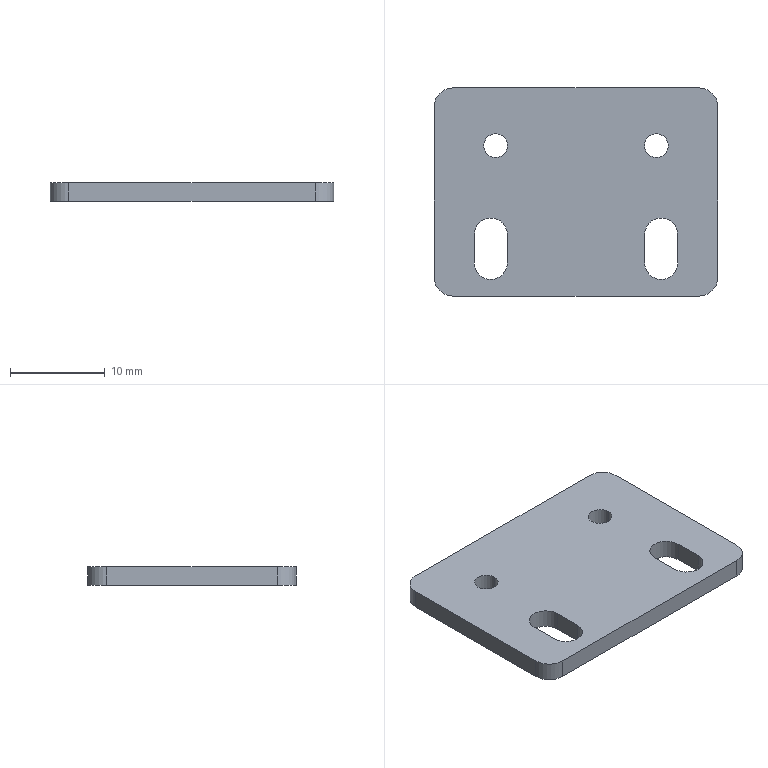Part | SolidWorks | features Cut 1, Fillet 1, FlatPattern 1, HoleWzd 1, SMBaseFlange 1, SheetMetal 1 | 1 solid | 22 faces | box 30 x 22 x 2 mm | volume 1213 mm3 | cylinder 12 | plane 10 | commonest cylinder face diameters 2.5 x4 3.5 x4 4 x4
STEP:
#1=CARTESIAN_POINT('',(-7.25,4.9,0.));
#2=VERTEX_POINT('',#1);
#3=CARTESIAN_POINT('',(-9.75,4.9,0.));
#4=VERTEX_POINT('',#3);
#5=CARTESIAN_POINT('',(-8.5,4.9,0.));
#6=DIRECTION('',(0.,0.,-1.));
#7=DIRECTION('',(-1.,0.,0.));
#8=AXIS2_PLACEMENT_3D('',#5,#6,#7);
#9=CIRCLE('',#8,1.25);
#10=EDGE_CURVE('',#2,#4,#9,.T.);
#11=ORIENTED_EDGE('',*,*,#10,.F.);
#12=CARTESIAN_POINT('',(-7.25,4.9,-2.));
#13=VERTEX_POINT('',#12);
#14=CARTESIAN_POINT('',(-7.25,4.9,-2.));
#15=DIRECTION('',(0.,0.,-1.));
#16=VECTOR('',#15,1000.);
#17=LINE('',#14,#16);
#18=EDGE_CURVE('',#2,#13,#17,.T.);
#19=ORIENTED_EDGE('',*,*,#18,.T.);
#20=CARTESIAN_POINT('',(-9.75,4.9,-2.));
#21=VERTEX_POINT('',#20);
#22=CARTESIAN_POINT('',(-8.5,4.9,-2.));
#23=DIRECTION('',(0.,0.,-1.));
#24=DIRECTION('',(-1.,0.,0.));
#25=AXIS2_PLACEMENT_3D('',#22,#23,#24);
#26=CIRCLE('',#25,1.25);
#27=EDGE_CURVE('',#13,#21,#26,.T.);
#28=ORIENTED_EDGE('',*,*,#27,.T.);
#29=CARTESIAN_POINT('',(-9.75,4.9,-2.));
#30=DIRECTION('',(0.,0.,-1.));
#31=VECTOR('',#30,1000.);
#32=LINE('',#29,#31);
#33=EDGE_CURVE('',#4,#21,#32,.T.);
#34=ORIENTED_EDGE('',*,*,#33,.F.);
#35=EDGE_LOOP('',(#11,#19,#28,#34));
#36=FACE_OUTER_BOUND('',#35,.T.);
#37=CARTESIAN_POINT('',(-8.5,4.9,-2.));
#38=DIRECTION('',(0.,0.,-1.));
#39=DIRECTION('',(-1.,0.,0.));
#40=AXIS2_PLACEMENT_3D('',#37,#38,#39);
#41=CYLINDRICAL_SURFACE('',#40,1.25);
#42=ADVANCED_FACE('',(#36),#41,.F.);
#43=CARTESIAN_POINT('',(9.75,4.9,0.));
#44=VERTEX_POINT('',#43);
#45=CARTESIAN_POINT('',(7.25,4.9,0.));
#46=VERTEX_POINT('',#45);
#47=CARTESIAN_POINT('',(8.5,4.9,0.));
#48=DIRECTION('',(0.,0.,-1.));
#49=DIRECTION('',(-1.,0.,0.));
#50=AXIS2_PLACEMENT_3D('',#47,#48,#49);
#51=CIRCLE('',#50,1.25);
#52=EDGE_CURVE('',#44,#46,#51,.T.);
#53=ORIENTED_EDGE('',*,*,#52,.F.);
#54=CARTESIAN_POINT('',(9.75,4.9,-2.));
#55=VERTEX_POINT('',#54);
#56=CARTESIAN_POINT('',(9.75,4.9,-2.));
#57=DIRECTION('',(0.,0.,-1.));
#58=VECTOR('',#57,1000.);
#59=LINE('',#56,#58);
#60=EDGE_CURVE('',#44,#55,#59,.T.);
#61=ORIENTED_EDGE('',*,*,#60,.T.);
#62=CARTESIAN_POINT('',(7.25,4.9,-2.));
#63=VERTEX_POINT('',#62);
#64=CARTESIAN_POINT('',(8.5,4.9,-2.));
#65=DIRECTION('',(0.,0.,-1.));
#66=DIRECTION('',(-1.,0.,0.));
#67=AXIS2_PLACEMENT_3D('',#64,#65,#66);
#68=CIRCLE('',#67,1.25);
#69=EDGE_CURVE('',#55,#63,#68,.T.);
#70=ORIENTED_EDGE('',*,*,#69,.T.);
#71=CARTESIAN_POINT('',(7.25,4.9,-2.));
#72=DIRECTION('',(0.,0.,-1.));
#73=VECTOR('',#72,1000.);
#74=LINE('',#71,#73);
#75=EDGE_CURVE('',#46,#63,#74,.T.);
#76=ORIENTED_EDGE('',*,*,#75,.F.);
#77=EDGE_LOOP('',(#53,#61,#70,#76));
#78=FACE_OUTER_BOUND('',#77,.T.);
#79=CARTESIAN_POINT('',(8.5,4.9,-2.));
#80=DIRECTION('',(0.,0.,-1.));
#81=DIRECTION('',(-1.,0.,0.));
#82=AXIS2_PLACEMENT_3D('',#79,#80,#81);
#83=CYLINDRICAL_SURFACE('',#82,1.25);
#84=ADVANCED_FACE('',(#78),#83,.F.);
#85=CARTESIAN_POINT('',(15.,-9.,-2.));
#86=VERTEX_POINT('',#85);
#87=CARTESIAN_POINT('',(15.,9.,-2.));
#88=VERTEX_POINT('',#87);
#89=CARTESIAN_POINT('',(15.,-11.,-2.));
#90=DIRECTION('',(0.,1.,0.));
#91=VECTOR('',#90,1000.);
#92=LINE('',#89,#91);
#93=EDGE_CURVE('',#86,#88,#92,.T.);
#94=ORIENTED_EDGE('',*,*,#93,.T.);
#95=CARTESIAN_POINT('',(15.,9.,0.));
#96=VERTEX_POINT('',#95);
#97=CARTESIAN_POINT('',(15.,9.,-2.));
#98=DIRECTION('',(0.,0.,1.));
#99=VECTOR('',#98,1000.);
#100=LINE('',#97,#99);
#101=EDGE_CURVE('',#88,#96,#100,.T.);
#102=ORIENTED_EDGE('',*,*,#101,.T.);
#103=CARTESIAN_POINT('',(15.,-9.,0.));
#104=VERTEX_POINT('',#103);
#105=CARTESIAN_POINT('',(15.,-11.,0.));
#106=DIRECTION('',(0.,1.,0.));
#107=VECTOR('',#106,1000.);
#108=LINE('',#105,#107);
#109=EDGE_CURVE('',#104,#96,#108,.T.);
#110=ORIENTED_EDGE('',*,*,#109,.F.);
#111=CARTESIAN_POINT('',(15.,-9.,-2.));
#112=DIRECTION('',(0.,0.,-1.));
#113=VECTOR('',#112,1000.);
#114=LINE('',#111,#113);
#115=EDGE_CURVE('',#104,#86,#114,.T.);
#116=ORIENTED_EDGE('',*,*,#115,.T.);
#117=EDGE_LOOP('',(#94,#102,#110,#116));
#118=FACE_OUTER_BOUND('',#117,.T.);
#119=CARTESIAN_POINT('',(15.,-11.,-2.));
#120=DIRECTION('',(1.,0.,0.));
#121=DIRECTION('',(0.,0.,-1.));
#122=AXIS2_PLACEMENT_3D('',#119,#120,#121);
#123=PLANE('',#122);
#124=ADVANCED_FACE('',(#118),#123,.T.);
#125=CARTESIAN_POINT('',(-13.,-11.,0.));
#126=VERTEX_POINT('',#125);
#127=CARTESIAN_POINT('',(13.,-11.,0.));
#128=VERTEX_POINT('',#127);
#129=CARTESIAN_POINT('',(-15.,-11.,0.));
#130=DIRECTION('',(1.,0.,0.));
#131=VECTOR('',#130,1000.);
#132=LINE('',#129,#131);
#133=EDGE_CURVE('',#126,#128,#132,.T.);
#134=ORIENTED_EDGE('',*,*,#133,.F.);
#135=CARTESIAN_POINT('',(-13.,-11.,-2.));
#136=VERTEX_POINT('',#135);
#137=CARTESIAN_POINT('',(-13.,-11.,-2.));
#138=DIRECTION('',(0.,0.,-1.));
#139=VECTOR('',#138,1000.);
#140=LINE('',#137,#139);
#141=EDGE_CURVE('',#126,#136,#140,.T.);
#142=ORIENTED_EDGE('',*,*,#141,.T.);
#143=CARTESIAN_POINT('',(13.,-11.,-2.));
#144=VERTEX_POINT('',#143);
#145=CARTESIAN_POINT('',(-15.,-11.,-2.));
#146=DIRECTION('',(1.,0.,0.));
#147=VECTOR('',#146,1000.);
#148=LINE('',#145,#147);
#149=EDGE_CURVE('',#136,#144,#148,.T.);
#150=ORIENTED_EDGE('',*,*,#149,.T.);
#151=CARTESIAN_POINT('',(13.,-11.,-2.));
#152=DIRECTION('',(0.,0.,1.));
#153=VECTOR('',#152,1000.);
#154=LINE('',#151,#153);
#155=EDGE_CURVE('',#144,#128,#154,.T.);
#156=ORIENTED_EDGE('',*,*,#155,.T.);
#157=EDGE_LOOP('',(#134,#142,#150,#156));
#158=FACE_OUTER_BOUND('',#157,.T.);
#159=CARTESIAN_POINT('',(-15.,-11.,-2.));
#160=DIRECTION('',(0.,-1.,0.));
#161=DIRECTION('',(0.,0.,-1.));
#162=AXIS2_PLACEMENT_3D('',#159,#160,#161);
#163=PLANE('',#162);
#164=ADVANCED_FACE('',(#158),#163,.T.);
#165=CARTESIAN_POINT('',(-15.,9.,-2.));
#166=VERTEX_POINT('',#165);
#167=CARTESIAN_POINT('',(-15.,-9.,-2.));
#168=VERTEX_POINT('',#167);
#169=CARTESIAN_POINT('',(-15.,-11.,-2.));
#170=DIRECTION('',(0.,-1.,0.));
#171=VECTOR('',#170,1000.);
#172=LINE('',#169,#171);
#173=EDGE_CURVE('',#166,#168,#172,.T.);
#174=ORIENTED_EDGE('',*,*,#173,.T.);
#175=CARTESIAN_POINT('',(-15.,-9.,0.));
#176=VERTEX_POINT('',#175);
#177=CARTESIAN_POINT('',(-15.,-9.,-2.));
#178=DIRECTION('',(0.,0.,1.));
#179=VECTOR('',#178,1000.);
#180=LINE('',#177,#179);
#181=EDGE_CURVE('',#168,#176,#180,.T.);
#182=ORIENTED_EDGE('',*,*,#181,.T.);
#183=CARTESIAN_POINT('',(-15.,9.,0.));
#184=VERTEX_POINT('',#183);
#185=CARTESIAN_POINT('',(-15.,-11.,0.));
#186=DIRECTION('',(0.,-1.,0.));
#187=VECTOR('',#186,1000.);
#188=LINE('',#185,#187);
#189=EDGE_CURVE('',#184,#176,#188,.T.);
#190=ORIENTED_EDGE('',*,*,#189,.F.);
#191=CARTESIAN_POINT('',(-15.,9.,-2.));
#192=DIRECTION('',(0.,0.,-1.));
#193=VECTOR('',#192,1000.);
#194=LINE('',#191,#193);
#195=EDGE_CURVE('',#184,#166,#194,.T.);
#196=ORIENTED_EDGE('',*,*,#195,.T.);
#197=EDGE_LOOP('',(#174,#182,#190,#196));
#198=FACE_OUTER_BOUND('',#197,.T.);
#199=CARTESIAN_POINT('',(-15.,-11.,-2.));
#200=DIRECTION('',(-1.,0.,0.));
#201=DIRECTION('',(0.,0.,1.));
#202=AXIS2_PLACEMENT_3D('',#199,#200,#201);
#203=PLANE('',#202);
#204=ADVANCED_FACE('',(#198),#203,.T.);
#205=CARTESIAN_POINT('',(13.,11.,-2.));
#206=VERTEX_POINT('',#205);
#207=CARTESIAN_POINT('',(-13.,11.,-2.));
#208=VERTEX_POINT('',#207);
#209=CARTESIAN_POINT('',(-15.,11.,-2.));
#210=DIRECTION('',(-1.,0.,0.));
#211=VECTOR('',#210,1000.);
#212=LINE('',#209,#211);
#213=EDGE_CURVE('',#206,#208,#212,.T.);
#214=ORIENTED_EDGE('',*,*,#213,.T.);
#215=CARTESIAN_POINT('',(-13.,11.,0.));
#216=VERTEX_POINT('',#215);
#217=CARTESIAN_POINT('',(-13.,11.,-2.));
#218=DIRECTION('',(0.,0.,1.));
#219=VECTOR('',#218,1000.);
#220=LINE('',#217,#219);
#221=EDGE_CURVE('',#208,#216,#220,.T.);
#222=ORIENTED_EDGE('',*,*,#221,.T.);
#223=CARTESIAN_POINT('',(13.,11.,0.));
#224=VERTEX_POINT('',#223);
#225=CARTESIAN_POINT('',(-15.,11.,0.));
#226=DIRECTION('',(-1.,0.,0.));
#227=VECTOR('',#226,1000.);
#228=LINE('',#225,#227);
#229=EDGE_CURVE('',#224,#216,#228,.T.);
#230=ORIENTED_EDGE('',*,*,#229,.F.);
#231=CARTESIAN_POINT('',(13.,11.,-2.));
#232=DIRECTION('',(0.,0.,-1.));
#233=VECTOR('',#232,1000.);
#234=LINE('',#231,#233);
#235=EDGE_CURVE('',#224,#206,#234,.T.);
#236=ORIENTED_EDGE('',*,*,#235,.T.);
#237=EDGE_LOOP('',(#214,#222,#230,#236));
#238=FACE_OUTER_BOUND('',#237,.T.);
#239=CARTESIAN_POINT('',(-15.,11.,-2.));
#240=DIRECTION('',(0.,1.,0.));
#241=DIRECTION('',(0.,0.,1.));
#242=AXIS2_PLACEMENT_3D('',#239,#240,#241);
#243=PLANE('',#242);
#244=ADVANCED_FACE('',(#238),#243,.T.);
#245=CARTESIAN_POINT('',(-8.5,4.9,-2.));
#246=DIRECTION('',(0.,0.,-1.));
#247=DIRECTION('',(-1.,0.,0.));
#248=AXIS2_PLACEMENT_3D('',#245,#246,#247);
#249=CIRCLE('',#248,1.25);
#250=EDGE_CURVE('',#21,#13,#249,.T.);
#251=ORIENTED_EDGE('',*,*,#250,.F.);
#252=ORIENTED_EDGE('',*,*,#27,.F.);
#253=EDGE_LOOP('',(#251,#252));
#254=FACE_BOUND('',#253,.T.);
#255=CARTESIAN_POINT('',(8.5,4.9,-2.));
#256=DIRECTION('',(0.,0.,-1.));
#257=DIRECTION('',(-1.,0.,0.));
#258=AXIS2_PLACEMENT_3D('',#255,#256,#257);
#259=CIRCLE('',#258,1.25);
#260=EDGE_CURVE('',#63,#55,#259,.T.);
#261=ORIENTED_EDGE('',*,*,#260,.F.);
#262=ORIENTED_EDGE('',*,*,#69,.F.);
#263=EDGE_LOOP('',(#261,#262));
#264=FACE_BOUND('',#263,.T.);
#265=CARTESIAN_POINT('',(7.25,-4.5,-2.));
#266=VERTEX_POINT('',#265);
#267=CARTESIAN_POINT('',(10.75,-4.5,-2.));
#268=VERTEX_POINT('',#267);
#269=CARTESIAN_POINT('',(9.,-4.5,-2.));
#270=DIRECTION('',(0.,0.,-1.));
#271=DIRECTION('',(-1.,0.,0.));
#272=AXIS2_PLACEMENT_3D('',#269,#270,#271);
#273=CIRCLE('',#272,1.75);
#274=EDGE_CURVE('',#266,#268,#273,.T.);
#275=ORIENTED_EDGE('',*,*,#274,.F.);
#276=CARTESIAN_POINT('',(7.25,-7.5,-2.));
#277=VERTEX_POINT('',#276);
#278=CARTESIAN_POINT('',(7.25,-4.5,-2.));
#279=DIRECTION('',(0.,1.,0.));
#280=VECTOR('',#279,1000.);
#281=LINE('',#278,#280);
#282=EDGE_CURVE('',#277,#266,#281,.T.);
#283=ORIENTED_EDGE('',*,*,#282,.F.);
#284=CARTESIAN_POINT('',(10.75,-7.5,-2.));
#285=VERTEX_POINT('',#284);
#286=CARTESIAN_POINT('',(9.,-7.5,-2.));
#287=DIRECTION('',(0.,0.,-1.));
#288=DIRECTION('',(-1.,0.,0.));
#289=AXIS2_PLACEMENT_3D('',#286,#287,#288);
#290=CIRCLE('',#289,1.75);
#291=EDGE_CURVE('',#285,#277,#290,.T.);
#292=ORIENTED_EDGE('',*,*,#291,.F.);
#293=CARTESIAN_POINT('',(10.75,-4.5,-2.));
#294=DIRECTION('',(0.,-1.,0.));
#295=VECTOR('',#294,1000.);
#296=LINE('',#293,#295);
#297=EDGE_CURVE('',#268,#285,#296,.T.);
#298=ORIENTED_EDGE('',*,*,#297,.F.);
#299=EDGE_LOOP('',(#275,#283,#292,#298));
#300=FACE_BOUND('',#299,.T.);
#301=CARTESIAN_POINT('',(-10.75,-4.5,-2.));
#302=VERTEX_POINT('',#301);
#303=CARTESIAN_POINT('',(-7.25,-4.5,-2.));
#304=VERTEX_POINT('',#303);
#305=CARTESIAN_POINT('',(-9.,-4.5,-2.));
#306=DIRECTION('',(0.,0.,-1.));
#307=DIRECTION('',(-1.,0.,0.));
#308=AXIS2_PLACEMENT_3D('',#305,#306,#307);
#309=CIRCLE('',#308,1.75);
#310=EDGE_CURVE('',#302,#304,#309,.T.);
#311=ORIENTED_EDGE('',*,*,#310,.F.);
#312=CARTESIAN_POINT('',(-10.75,-7.5,-2.));
#313=VERTEX_POINT('',#312);
#314=CARTESIAN_POINT('',(-10.75,-4.5,-2.));
#315=DIRECTION('',(0.,1.,0.));
#316=VECTOR('',#315,1000.);
#317=LINE('',#314,#316);
#318=EDGE_CURVE('',#313,#302,#317,.T.);
#319=ORIENTED_EDGE('',*,*,#318,.F.);
#320=CARTESIAN_POINT('',(-7.25,-7.5,-2.));
#321=VERTEX_POINT('',#320);
#322=CARTESIAN_POINT('',(-9.,-7.5,-2.));
#323=DIRECTION('',(0.,0.,-1.));
#324=DIRECTION('',(-1.,0.,0.));
#325=AXIS2_PLACEMENT_3D('',#322,#323,#324);
#326=CIRCLE('',#325,1.75);
#327=EDGE_CURVE('',#321,#313,#326,.T.);
#328=ORIENTED_EDGE('',*,*,#327,.F.);
#329=CARTESIAN_POINT('',(-7.25,-4.5,-2.));
#330=DIRECTION('',(0.,-1.,0.));
#331=VECTOR('',#330,1000.);
#332=LINE('',#329,#331);
#333=EDGE_CURVE('',#304,#321,#332,.T.);
#334=ORIENTED_EDGE('',*,*,#333,.F.);
#335=EDGE_LOOP('',(#311,#319,#328,#334));
#336=FACE_BOUND('',#335,.T.);
#337=ORIENTED_EDGE('',*,*,#149,.F.);
#338=CARTESIAN_POINT('',(-13.,-9.,-2.));
#339=DIRECTION('',(0.,0.,-1.));
#340=DIRECTION('',(-1.,0.,0.));
#341=AXIS2_PLACEMENT_3D('',#338,#339,#340);
#342=CIRCLE('',#341,2.);
#343=EDGE_CURVE('',#136,#168,#342,.T.);
#344=ORIENTED_EDGE('',*,*,#343,.T.);
#345=ORIENTED_EDGE('',*,*,#173,.F.);
#346=CARTESIAN_POINT('',(-13.,9.,-2.));
#347=DIRECTION('',(0.,0.,-1.));
#348=DIRECTION('',(-1.,0.,0.));
#349=AXIS2_PLACEMENT_3D('',#346,#347,#348);
#350=CIRCLE('',#349,2.);
#351=EDGE_CURVE('',#166,#208,#350,.T.);
#352=ORIENTED_EDGE('',*,*,#351,.T.);
#353=ORIENTED_EDGE('',*,*,#213,.F.);
#354=CARTESIAN_POINT('',(13.,9.,-2.));
#355=DIRECTION('',(0.,0.,-1.));
#356=DIRECTION('',(-1.,0.,0.));
#357=AXIS2_PLACEMENT_3D('',#354,#355,#356);
#358=CIRCLE('',#357,2.);
#359=EDGE_CURVE('',#206,#88,#358,.T.);
#360=ORIENTED_EDGE('',*,*,#359,.T.);
#361=ORIENTED_EDGE('',*,*,#93,.F.);
#362=CARTESIAN_POINT('',(13.,-9.,-2.));
#363=DIRECTION('',(0.,0.,-1.));
#364=DIRECTION('',(-1.,0.,0.));
#365=AXIS2_PLACEMENT_3D('',#362,#363,#364);
#366=CIRCLE('',#365,2.);
#367=EDGE_CURVE('',#86,#144,#366,.T.);
#368=ORIENTED_EDGE('',*,*,#367,.T.);
#369=EDGE_LOOP('',(#337,#344,#345,#352,#353,#360,#361,#368));
#370=FACE_OUTER_BOUND('',#369,.T.);
#371=CARTESIAN_POINT('',(0.,0.,-2.));
#372=DIRECTION('',(0.,0.,-1.));
#373=DIRECTION('',(-1.,0.,0.));
#374=AXIS2_PLACEMENT_3D('',#371,#372,#373);
#375=PLANE('',#374);
#376=ADVANCED_FACE('',(#254,#264,#300,#336,#370),#375,.T.);
#377=CARTESIAN_POINT('',(-8.5,4.9,0.));
#378=DIRECTION('',(0.,0.,-1.));
#379=DIRECTION('',(-1.,0.,0.));
#380=AXIS2_PLACEMENT_3D('',#377,#378,#379);
#381=CIRCLE('',#380,1.25);
#382=EDGE_CURVE('',#4,#2,#381,.T.);
#383=ORIENTED_EDGE('',*,*,#382,.T.);
#384=ORIENTED_EDGE('',*,*,#10,.T.);
#385=EDGE_LOOP('',(#383,#384));
#386=FACE_BOUND('',#385,.T.);
#387=CARTESIAN_POINT('',(8.5,4.9,0.));
#388=DIRECTION('',(0.,0.,-1.));
#389=DIRECTION('',(-1.,0.,0.));
#390=AXIS2_PLACEMENT_3D('',#387,#388,#389);
#391=CIRCLE('',#390,1.25);
#392=EDGE_CURVE('',#46,#44,#391,.T.);
#393=ORIENTED_EDGE('',*,*,#392,.T.);
#394=ORIENTED_EDGE('',*,*,#52,.T.);
#395=EDGE_LOOP('',(#393,#394));
#396=FACE_BOUND('',#395,.T.);
#397=CARTESIAN_POINT('',(7.25,-7.5,0.));
#398=VERTEX_POINT('',#397);
#399=CARTESIAN_POINT('',(7.25,-4.5,0.));
#400=VERTEX_POINT('',#399);
#401=CARTESIAN_POINT('',(7.25,-4.5,0.));
#402=DIRECTION('',(0.,1.,0.));
#403=VECTOR('',#402,1000.);
#404=LINE('',#401,#403);
#405=EDGE_CURVE('',#398,#400,#404,.T.);
#406=ORIENTED_EDGE('',*,*,#405,.T.);
#407=CARTESIAN_POINT('',(10.75,-4.5,0.));
#408=VERTEX_POINT('',#407);
#409=CARTESIAN_POINT('',(9.,-4.5,0.));
#410=DIRECTION('',(0.,0.,-1.));
#411=DIRECTION('',(-1.,0.,0.));
#412=AXIS2_PLACEMENT_3D('',#409,#410,#411);
#413=CIRCLE('',#412,1.75);
#414=EDGE_CURVE('',#400,#408,#413,.T.);
#415=ORIENTED_EDGE('',*,*,#414,.T.);
#416=CARTESIAN_POINT('',(10.75,-7.5,0.));
#417=VERTEX_POINT('',#416);
#418=CARTESIAN_POINT('',(10.75,-4.5,0.));
#419=DIRECTION('',(0.,-1.,0.));
#420=VECTOR('',#419,1000.);
#421=LINE('',#418,#420);
#422=EDGE_CURVE('',#408,#417,#421,.T.);
#423=ORIENTED_EDGE('',*,*,#422,.T.);
#424=CARTESIAN_POINT('',(9.,-7.5,0.));
#425=DIRECTION('',(0.,0.,-1.));
#426=DIRECTION('',(-1.,0.,0.));
#427=AXIS2_PLACEMENT_3D('',#424,#425,#426);
#428=CIRCLE('',#427,1.75);
#429=EDGE_CURVE('',#417,#398,#428,.T.);
#430=ORIENTED_EDGE('',*,*,#429,.T.);
#431=EDGE_LOOP('',(#406,#415,#423,#430));
#432=FACE_BOUND('',#431,.T.);
#433=CARTESIAN_POINT('',(-10.75,-7.5,0.));
#434=VERTEX_POINT('',#433);
#435=CARTESIAN_POINT('',(-10.75,-4.5,0.));
#436=VERTEX_POINT('',#435);
#437=CARTESIAN_POINT('',(-10.75,-4.5,0.));
#438=DIRECTION('',(0.,1.,0.));
#439=VECTOR('',#438,1000.);
#440=LINE('',#437,#439);
#441=EDGE_CURVE('',#434,#436,#440,.T.);
#442=ORIENTED_EDGE('',*,*,#441,.T.);
#443=CARTESIAN_POINT('',(-7.25,-4.5,0.));
#444=VERTEX_POINT('',#443);
#445=CARTESIAN_POINT('',(-9.,-4.5,0.));
#446=DIRECTION('',(0.,0.,-1.));
#447=DIRECTION('',(-1.,0.,0.));
#448=AXIS2_PLACEMENT_3D('',#445,#446,#447);
#449=CIRCLE('',#448,1.75);
#450=EDGE_CURVE('',#436,#444,#449,.T.);
#451=ORIENTED_EDGE('',*,*,#450,.T.);
#452=CARTESIAN_POINT('',(-7.25,-7.5,0.));
#453=VERTEX_POINT('',#452);
#454=CARTESIAN_POINT('',(-7.25,-4.5,0.));
#455=DIRECTION('',(0.,-1.,0.));
#456=VECTOR('',#455,1000.);
#457=LINE('',#454,#456);
#458=EDGE_CURVE('',#444,#453,#457,.T.);
#459=ORIENTED_EDGE('',*,*,#458,.T.);
#460=CARTESIAN_POINT('',(-9.,-7.5,0.));
#461=DIRECTION('',(0.,0.,-1.));
#462=DIRECTION('',(-1.,0.,0.));
#463=AXIS2_PLACEMENT_3D('',#460,#461,#462);
#464=CIRCLE('',#463,1.75);
#465=EDGE_CURVE('',#453,#434,#464,.T.);
#466=ORIENTED_EDGE('',*,*,#465,.T.);
#467=EDGE_LOOP('',(#442,#451,#459,#466));
#468=FACE_BOUND('',#467,.T.);
#469=ORIENTED_EDGE('',*,*,#189,.T.);
#470=CARTESIAN_POINT('',(-13.,-9.,0.));
#471=DIRECTION('',(0.,0.,1.));
#472=DIRECTION('',(-1.,0.,0.));
#473=AXIS2_PLACEMENT_3D('',#470,#471,#472);
#474=CIRCLE('',#473,2.);
#475=EDGE_CURVE('',#176,#126,#474,.T.);
#476=ORIENTED_EDGE('',*,*,#475,.T.);
#477=ORIENTED_EDGE('',*,*,#133,.T.);
#478=CARTESIAN_POINT('',(13.,-9.,0.));
#479=DIRECTION('',(0.,0.,1.));
#480=DIRECTION('',(-1.,0.,0.));
#481=AXIS2_PLACEMENT_3D('',#478,#479,#480);
#482=CIRCLE('',#481,2.);
#483=EDGE_CURVE('',#128,#104,#482,.T.);
#484=ORIENTED_EDGE('',*,*,#483,.T.);
#485=ORIENTED_EDGE('',*,*,#109,.T.);
#486=CARTESIAN_POINT('',(13.,9.,0.));
#487=DIRECTION('',(0.,0.,1.));
#488=DIRECTION('',(-1.,0.,0.));
#489=AXIS2_PLACEMENT_3D('',#486,#487,#488);
#490=CIRCLE('',#489,2.);
#491=EDGE_CURVE('',#96,#224,#490,.T.);
#492=ORIENTED_EDGE('',*,*,#491,.T.);
#493=ORIENTED_EDGE('',*,*,#229,.T.);
#494=CARTESIAN_POINT('',(-13.,9.,0.));
#495=DIRECTION('',(0.,0.,1.));
#496=DIRECTION('',(-1.,0.,0.));
#497=AXIS2_PLACEMENT_3D('',#494,#495,#496);
#498=CIRCLE('',#497,2.);
#499=EDGE_CURVE('',#216,#184,#498,.T.);
#500=ORIENTED_EDGE('',*,*,#499,.T.);
#501=EDGE_LOOP('',(#469,#476,#477,#484,#485,#492,#493,#500));
#502=FACE_OUTER_BOUND('',#501,.T.);
#503=CARTESIAN_POINT('',(0.,0.,0.));
#504=DIRECTION('',(0.,0.,-1.));
#505=DIRECTION('',(-1.,0.,0.));
#506=AXIS2_PLACEMENT_3D('',#503,#504,#505);
#507=PLANE('',#506);
#508=ADVANCED_FACE('',(#386,#396,#432,#468,#502),#507,.F.);
#509=ORIENTED_EDGE('',*,*,#310,.T.);
#510=CARTESIAN_POINT('',(-7.25,-4.5,0.));
#511=DIRECTION('',(0.,0.,-1.));
#512=VECTOR('',#511,1000.);
#513=LINE('',#510,#512);
#514=EDGE_CURVE('',#444,#304,#513,.T.);
#515=ORIENTED_EDGE('',*,*,#514,.F.);
#516=ORIENTED_EDGE('',*,*,#450,.F.);
#517=CARTESIAN_POINT('',(-10.75,-4.5,0.));
#518=DIRECTION('',(0.,0.,-1.));
#519=VECTOR('',#518,1000.);
#520=LINE('',#517,#519);
#521=EDGE_CURVE('',#436,#302,#520,.T.);
#522=ORIENTED_EDGE('',*,*,#521,.T.);
#523=EDGE_LOOP('',(#509,#515,#516,#522));
#524=FACE_OUTER_BOUND('',#523,.T.);
#525=CARTESIAN_POINT('',(-9.,-4.5,0.));
#526=DIRECTION('',(0.,0.,-1.));
#527=DIRECTION('',(-1.,0.,0.));
#528=AXIS2_PLACEMENT_3D('',#525,#526,#527);
#529=CYLINDRICAL_SURFACE('',#528,1.75);
#530=ADVANCED_FACE('',(#524),#529,.F.);
#531=ORIENTED_EDGE('',*,*,#318,.T.);
#532=ORIENTED_EDGE('',*,*,#521,.F.);
#533=ORIENTED_EDGE('',*,*,#441,.F.);
#534=CARTESIAN_POINT('',(-10.75,-7.5,0.));
#535=DIRECTION('',(0.,0.,-1.));
#536=VECTOR('',#535,1000.);
#537=LINE('',#534,#536);
#538=EDGE_CURVE('',#434,#313,#537,.T.);
#539=ORIENTED_EDGE('',*,*,#538,.T.);
#540=EDGE_LOOP('',(#531,#532,#533,#539));
#541=FACE_OUTER_BOUND('',#540,.T.);
#542=CARTESIAN_POINT('',(-10.75,-4.5,0.));
#543=DIRECTION('',(-1.,0.,0.));
#544=DIRECTION('',(0.,0.,1.));
#545=AXIS2_PLACEMENT_3D('',#542,#543,#544);
#546=PLANE('',#545);
#547=ADVANCED_FACE('',(#541),#546,.F.);
#548=ORIENTED_EDGE('',*,*,#327,.T.);
#549=ORIENTED_EDGE('',*,*,#538,.F.);
#550=ORIENTED_EDGE('',*,*,#465,.F.);
#551=CARTESIAN_POINT('',(-7.25,-7.5,0.));
#552=DIRECTION('',(0.,0.,-1.));
#553=VECTOR('',#552,1000.);
#554=LINE('',#551,#553);
#555=EDGE_CURVE('',#453,#321,#554,.T.);
#556=ORIENTED_EDGE('',*,*,#555,.T.);
#557=EDGE_LOOP('',(#548,#549,#550,#556));
#558=FACE_OUTER_BOUND('',#557,.T.);
#559=CARTESIAN_POINT('',(-9.,-7.5,0.));
#560=DIRECTION('',(0.,0.,-1.));
#561=DIRECTION('',(-1.,0.,0.));
#562=AXIS2_PLACEMENT_3D('',#559,#560,#561);
#563=CYLINDRICAL_SURFACE('',#562,1.75);
#564=ADVANCED_FACE('',(#558),#563,.F.);
#565=ORIENTED_EDGE('',*,*,#333,.T.);
#566=ORIENTED_EDGE('',*,*,#555,.F.);
#567=ORIENTED_EDGE('',*,*,#458,.F.);
#568=ORIENTED_EDGE('',*,*,#514,.T.);
#569=EDGE_LOOP('',(#565,#566,#567,#568));
#570=FACE_OUTER_BOUND('',#569,.T.);
#571=CARTESIAN_POINT('',(-7.25,-4.5,0.));
#572=DIRECTION('',(1.,0.,0.));
#573=DIRECTION('',(0.,0.,-1.));
#574=AXIS2_PLACEMENT_3D('',#571,#572,#573);
#575=PLANE('',#574);
#576=ADVANCED_FACE('',(#570),#575,.F.);
#577=ORIENTED_EDGE('',*,*,#274,.T.);
#578=CARTESIAN_POINT('',(10.75,-4.5,0.));
#579=DIRECTION('',(0.,0.,-1.));
#580=VECTOR('',#579,1000.);
#581=LINE('',#578,#580);
#582=EDGE_CURVE('',#408,#268,#581,.T.);
#583=ORIENTED_EDGE('',*,*,#582,.F.);
#584=ORIENTED_EDGE('',*,*,#414,.F.);
#585=CARTESIAN_POINT('',(7.25,-4.5,0.));
#586=DIRECTION('',(0.,0.,-1.));
#587=VECTOR('',#586,1000.);
#588=LINE('',#585,#587);
#589=EDGE_CURVE('',#400,#266,#588,.T.);
#590=ORIENTED_EDGE('',*,*,#589,.T.);
#591=EDGE_LOOP('',(#577,#583,#584,#590));
#592=FACE_OUTER_BOUND('',#591,.T.);
#593=CARTESIAN_POINT('',(9.,-4.5,0.));
#594=DIRECTION('',(0.,0.,-1.));
#595=DIRECTION('',(-1.,0.,0.));
#596=AXIS2_PLACEMENT_3D('',#593,#594,#595);
#597=CYLINDRICAL_SURFACE('',#596,1.75);
#598=ADVANCED_FACE('',(#592),#597,.F.);
#599=ORIENTED_EDGE('',*,*,#282,.T.);
#600=ORIENTED_EDGE('',*,*,#589,.F.);
#601=ORIENTED_EDGE('',*,*,#405,.F.);
#602=CARTESIAN_POINT('',(7.25,-7.5,0.));
#603=DIRECTION('',(0.,0.,-1.));
#604=VECTOR('',#603,1000.);
#605=LINE('',#602,#604);
#606=EDGE_CURVE('',#398,#277,#605,.T.);
#607=ORIENTED_EDGE('',*,*,#606,.T.);
#608=EDGE_LOOP('',(#599,#600,#601,#607));
#609=FACE_OUTER_BOUND('',#608,.T.);
#610=CARTESIAN_POINT('',(7.25,-4.5,0.));
#611=DIRECTION('',(-1.,0.,0.));
#612=DIRECTION('',(0.,0.,1.));
#613=AXIS2_PLACEMENT_3D('',#610,#611,#612);
#614=PLANE('',#613);
#615=ADVANCED_FACE('',(#609),#614,.F.);
#616=ORIENTED_EDGE('',*,*,#291,.T.);
#617=ORIENTED_EDGE('',*,*,#606,.F.);
#618=ORIENTED_EDGE('',*,*,#429,.F.);
#619=CARTESIAN_POINT('',(10.75,-7.5,0.));
#620=DIRECTION('',(0.,0.,-1.));
#621=VECTOR('',#620,1000.);
#622=LINE('',#619,#621);
#623=EDGE_CURVE('',#417,#285,#622,.T.);
#624=ORIENTED_EDGE('',*,*,#623,.T.);
#625=EDGE_LOOP('',(#616,#617,#618,#624));
#626=FACE_OUTER_BOUND('',#625,.T.);
#627=CARTESIAN_POINT('',(9.,-7.5,0.));
#628=DIRECTION('',(0.,0.,-1.));
#629=DIRECTION('',(-1.,0.,0.));
#630=AXIS2_PLACEMENT_3D('',#627,#628,#629);
#631=CYLINDRICAL_SURFACE('',#630,1.75);
#632=ADVANCED_FACE('',(#626),#631,.F.);
#633=ORIENTED_EDGE('',*,*,#297,.T.);
#634=ORIENTED_EDGE('',*,*,#623,.F.);
#635=ORIENTED_EDGE('',*,*,#422,.F.);
#636=ORIENTED_EDGE('',*,*,#582,.T.);
#637=EDGE_LOOP('',(#633,#634,#635,#636));
#638=FACE_OUTER_BOUND('',#637,.T.);
#639=CARTESIAN_POINT('',(10.75,-4.5,0.));
#640=DIRECTION('',(1.,0.,0.));
#641=DIRECTION('',(0.,0.,-1.));
#642=AXIS2_PLACEMENT_3D('',#639,#640,#641);
#643=PLANE('',#642);
#644=ADVANCED_FACE('',(#638),#643,.F.);
#645=ORIENTED_EDGE('',*,*,#60,.F.);
#646=ORIENTED_EDGE('',*,*,#392,.F.);
#647=ORIENTED_EDGE('',*,*,#75,.T.);
#648=ORIENTED_EDGE('',*,*,#260,.T.);
#649=EDGE_LOOP('',(#645,#646,#647,#648));
#650=FACE_OUTER_BOUND('',#649,.T.);
#651=CARTESIAN_POINT('',(8.5,4.9,-2.));
#652=DIRECTION('',(0.,0.,-1.));
#653=DIRECTION('',(-1.,0.,0.));
#654=AXIS2_PLACEMENT_3D('',#651,#652,#653);
#655=CYLINDRICAL_SURFACE('',#654,1.25);
#656=ADVANCED_FACE('',(#650),#655,.F.);
#657=ORIENTED_EDGE('',*,*,#18,.F.);
#658=ORIENTED_EDGE('',*,*,#382,.F.);
#659=ORIENTED_EDGE('',*,*,#33,.T.);
#660=ORIENTED_EDGE('',*,*,#250,.T.);
#661=EDGE_LOOP('',(#657,#658,#659,#660));
#662=FACE_OUTER_BOUND('',#661,.T.);
#663=CARTESIAN_POINT('',(-8.5,4.9,-2.));
#664=DIRECTION('',(0.,0.,-1.));
#665=DIRECTION('',(-1.,0.,0.));
#666=AXIS2_PLACEMENT_3D('',#663,#664,#665);
#667=CYLINDRICAL_SURFACE('',#666,1.25);
#668=ADVANCED_FACE('',(#662),#667,.F.);
#669=ORIENTED_EDGE('',*,*,#343,.F.);
#670=ORIENTED_EDGE('',*,*,#141,.F.);
#671=ORIENTED_EDGE('',*,*,#475,.F.);
#672=ORIENTED_EDGE('',*,*,#181,.F.);
#673=EDGE_LOOP('',(#669,#670,#671,#672));
#674=FACE_OUTER_BOUND('',#673,.T.);
#675=CARTESIAN_POINT('',(-13.,-9.,-2.));
#676=DIRECTION('',(0.,0.,1.));
#677=DIRECTION('',(1.,0.,0.));
#678=AXIS2_PLACEMENT_3D('',#675,#676,#677);
#679=CYLINDRICAL_SURFACE('',#678,2.);
#680=ADVANCED_FACE('',(#674),#679,.T.);
#681=ORIENTED_EDGE('',*,*,#351,.F.);
#682=ORIENTED_EDGE('',*,*,#195,.F.);
#683=ORIENTED_EDGE('',*,*,#499,.F.);
#684=ORIENTED_EDGE('',*,*,#221,.F.);
#685=EDGE_LOOP('',(#681,#682,#683,#684));
#686=FACE_OUTER_BOUND('',#685,.T.);
#687=CARTESIAN_POINT('',(-13.,9.,-2.));
#688=DIRECTION('',(0.,0.,1.));
#689=DIRECTION('',(1.,0.,0.));
#690=AXIS2_PLACEMENT_3D('',#687,#688,#689);
#691=CYLINDRICAL_SURFACE('',#690,2.);
#692=ADVANCED_FACE('',(#686),#691,.T.);
#693=ORIENTED_EDGE('',*,*,#359,.F.);
#694=ORIENTED_EDGE('',*,*,#235,.F.);
#695=ORIENTED_EDGE('',*,*,#491,.F.);
#696=ORIENTED_EDGE('',*,*,#101,.F.);
#697=EDGE_LOOP('',(#693,#694,#695,#696));
#698=FACE_OUTER_BOUND('',#697,.T.);
#699=CARTESIAN_POINT('',(13.,9.,-2.));
#700=DIRECTION('',(0.,0.,1.));
#701=DIRECTION('',(1.,0.,0.));
#702=AXIS2_PLACEMENT_3D('',#699,#700,#701);
#703=CYLINDRICAL_SURFACE('',#702,2.);
#704=ADVANCED_FACE('',(#698),#703,.T.);
#705=ORIENTED_EDGE('',*,*,#367,.F.);
#706=ORIENTED_EDGE('',*,*,#115,.F.);
#707=ORIENTED_EDGE('',*,*,#483,.F.);
#708=ORIENTED_EDGE('',*,*,#155,.F.);
#709=EDGE_LOOP('',(#705,#706,#707,#708));
#710=FACE_OUTER_BOUND('',#709,.T.);
#711=CARTESIAN_POINT('',(13.,-9.,-2.));
#712=DIRECTION('',(0.,0.,1.));
#713=DIRECTION('',(1.,0.,0.));
#714=AXIS2_PLACEMENT_3D('',#711,#712,#713);
#715=CYLINDRICAL_SURFACE('',#714,2.);
#716=ADVANCED_FACE('',(#710),#715,.T.);
#717=CLOSED_SHELL('',(#42,#84,#124,#164,#204,#244,#376,#508,#530,#547,#564,#576,#598,#615,#632,#644,#656,#668,#680,#692,#704,#716));
#718=MANIFOLD_SOLID_BREP('',#717);
#719=CARTESIAN_POINT('',(0.,0.,0.));
#720=DIRECTION('',(0.,0.,1.));
#721=DIRECTION('',(1.,0.,0.));
#722=AXIS2_PLACEMENT_3D('',#719,#720,#721);
#723=(LENGTH_UNIT()NAMED_UNIT(*)SI_UNIT(.MILLI.,.METRE.));
#724=UNCERTAINTY_MEASURE_WITH_UNIT(LENGTH_MEASURE(0.00001),#723,'','');
#725=(NAMED_UNIT(*)PLANE_ANGLE_UNIT()SI_UNIT($,.RADIAN.));
#726=(NAMED_UNIT(*)SI_UNIT($,.STERADIAN.)SOLID_ANGLE_UNIT());
#727=(GEOMETRIC_REPRESENTATION_CONTEXT(3)GLOBAL_UNCERTAINTY_ASSIGNED_CONTEXT((#724))GLOBAL_UNIT_ASSIGNED_CONTEXT((#723,#725,#726))REPRESENTATION_CONTEXT('',''));
#728=ADVANCED_BREP_SHAPE_REPRESENTATION('',(#718,#722),#727);